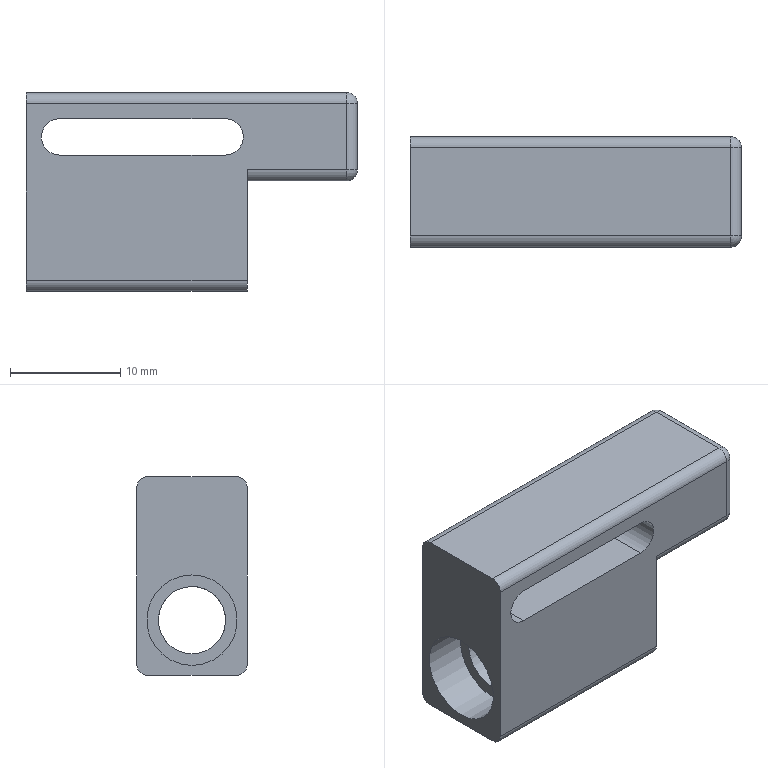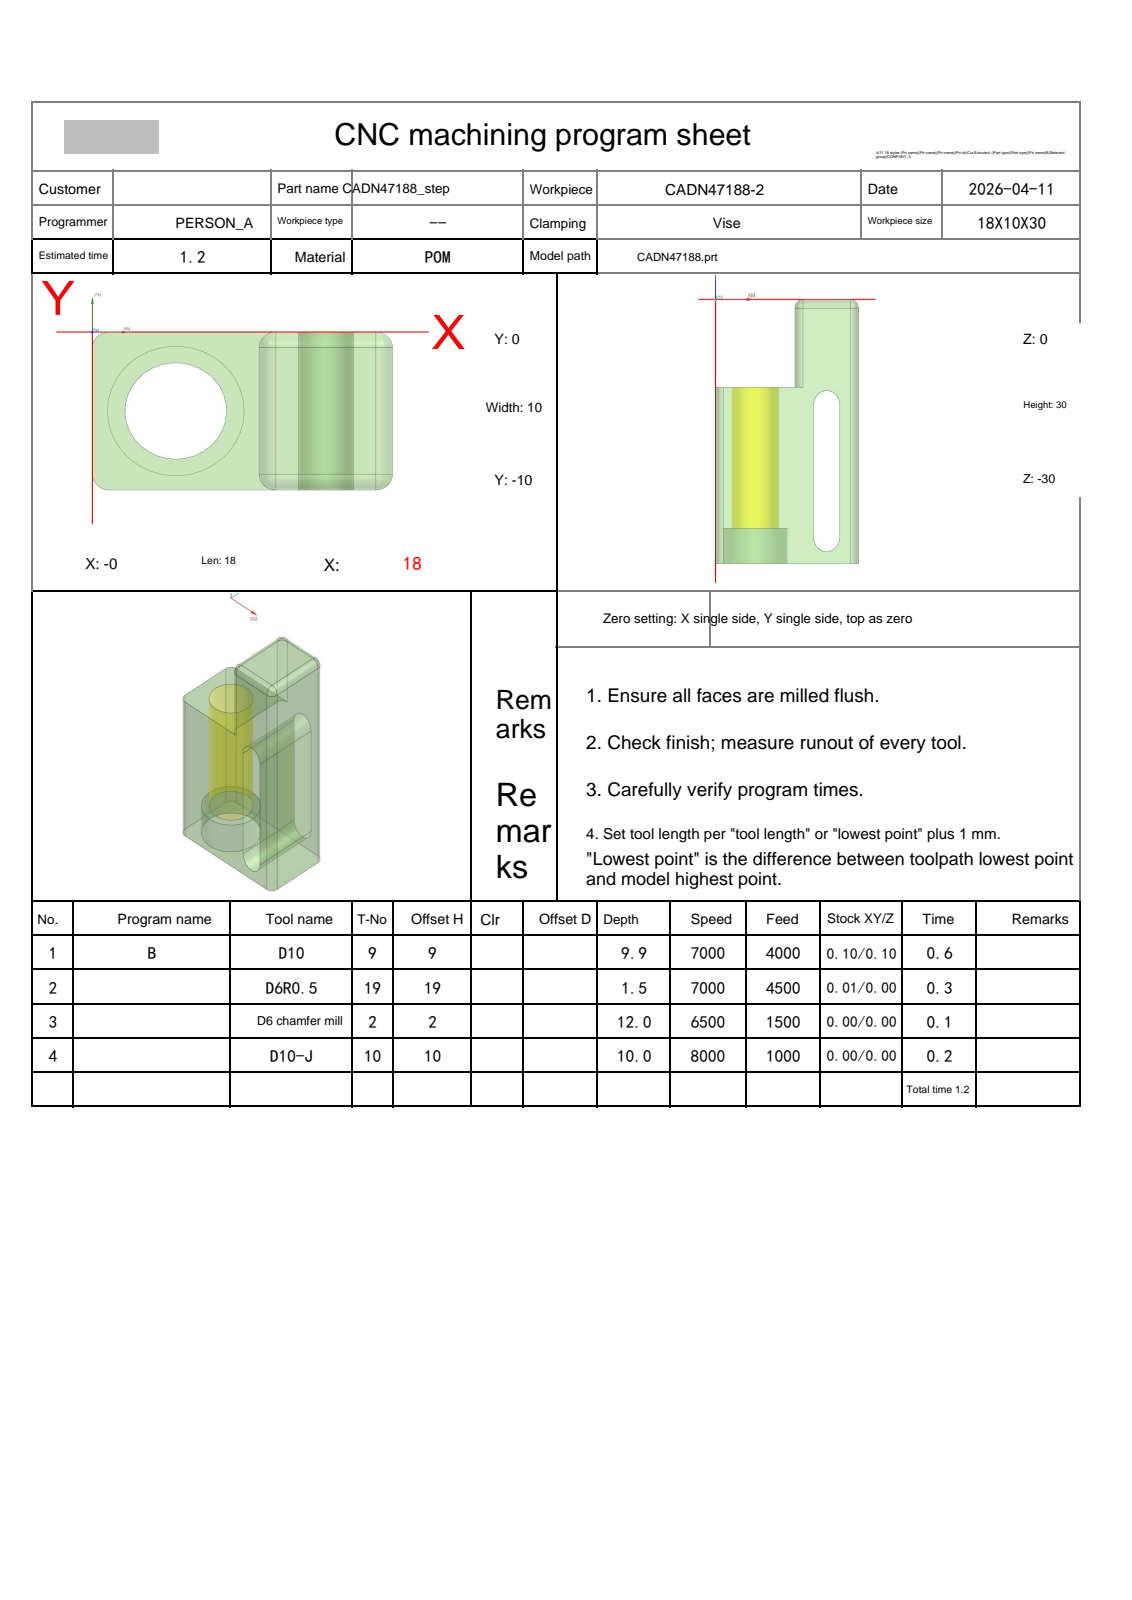NC program | NX | posted by the shop | part box 30 x 10 x 18 mm
Lines 457 to 1926 of 3974:
N2 T19 M06
(D6R0.5  D=6. R=0.5 H=19 ce=0.01 di=0.00)
G00 G90 G54 X13.171 Y-11.678 M03 S7000
G43 H19 Z20.
M08
Z1.5
G01 X10.836 Z1.378 F4500.
X10.409 Y-11.617 Z1.355
X9.997 Y-11.489 Z1.332
X9.611 Y-11.296 Z1.31
X9.261 Y-11.044 Z1.287
X8.956 Y-10.739 Z1.265
X8.704 Y-10.389 Z1.242
X8.511 Y-10.003 Z1.219
X8.383 Y-9.591 Z1.197
X8.322 Y-9.164 Z1.174
Y-.836 Z.738
X8.383 Y-.409 Z.715
X8.511 Y.003 Z.692
X8.704 Y.389 Z.67
X8.956 Y.739 Z.647
X9.261 Y1.044 Z.625
X9.611 Y1.296 Z.602
X9.997 Y1.489 Z.579
X10.409 Y1.617 Z.557
X10.836 Y1.678 Z.534
X17.164 Z.203
X17.591 Y1.617 Z.18
X18.003 Y1.489 Z.157
X18.389 Y1.296 Z.135
X18.739 Y1.044 Z.112
X19.044 Y.739 Z.09
X19.296 Y.389 Z.067
X19.489 Y.003 Z.044
X19.617 Y-.409 Z.022
X19.678 Y-.836 Z-.001
Y-1. Z-.009
Y-9.
G02 X17. Y-11.678 I-2.678 J0.0
G01 X11.
G02 X8.322 Y-9. I0.0 J2.678
G01 Y-1.
G02 X11. Y1.678 I2.678 J0.0
G01 X17.
G02 X19.678 Y-1. I0.0 J-2.678
G01 X19.684 Y-3. Z-.01
X19.69 Y-5. Z-.011
X19.695 Y-7. Z-.012
X19.701 Y-9.
X19.7 Y-9.082
X19.696 Y-9.163
X19.691 Y-9.245
X19.682 Y-9.326
X19.672 Y-9.407
X19.658 Y-9.487
X19.643 Y-9.567
X19.624 Y-9.647
X19.604 Y-9.726 Z-.013
X19.581 Y-9.804
X19.556 Y-9.882
X19.528 Y-9.959
X19.498 Y-10.035
X19.466 Y-10.11
X19.432 Y-10.184
X19.394 Y-10.257
X19.356 Y-10.329
X19.315 Y-10.399
X19.272 Y-10.469
X19.226 Y-10.537
X19.179 Y-10.604
X19.13 Y-10.668
X19.079 Y-10.733
X19.025 Y-10.794
X18.971 Y-10.855
X18.914 Y-10.914
X18.855 Y-10.971
X18.795 Y-11.026
X18.733 Y-11.08
X18.67 Y-11.131
X18.605 Y-11.181
X18.538 Y-11.228
X18.47 Y-11.274
X18.401 Y-11.317
X18.331 Y-11.359
X18.259 Y-11.398
X18.186 Y-11.436
X18.112 Y-11.47
X18.037 Y-11.503
X17.961 Y-11.533
X17.884 Y-11.562
X17.806 Y-11.587
X17.728 Y-11.611
X17.649 Y-11.631 Z-.014
X17.569 Y-11.651
X17.489 Y-11.666
X17.408 Y-11.68
X17.327 Y-11.691
X17.245 Y-11.701
X17.164 Y-11.706
X17.082 Y-11.711
X17. Y-11.712
X14. Y-11.72 Z-.015
X11. Y-11.727 Z-.016
X10.918 Y-11.726
X10.835 Y-11.723
X10.753 Y-11.717
X10.671 Y-11.708
X10.589 Y-11.697
X10.508 Y-11.684
X10.427 Y-11.668
X10.347 Y-11.65
X10.267 Y-11.629
X10.188 Y-11.606
X10.11 Y-11.58
X10.032 Y-11.552
X9.955 Y-11.522
X9.88 Y-11.49
X9.805 Y-11.455
X9.731 Y-11.418
X9.659 Y-11.378
X9.587 Y-11.337
X9.517 Y-11.293
X9.448 Y-11.248
X9.381 Y-11.2
X9.315 Y-11.15
X9.251 Y-11.099 Z-.017
X9.188 Y-11.045
X9.127 Y-10.989
X9.068 Y-10.932
X9.01 Y-10.873
X8.954 Y-10.812
X8.901 Y-10.75
X8.848 Y-10.686
X8.798 Y-10.62
X8.75 Y-10.553
X8.704 Y-10.484
X8.66 Y-10.414
X8.619 Y-10.343
X8.579 Y-10.271
X8.541 Y-10.197
X8.506 Y-10.122
X8.473 Y-10.047
X8.443 Y-9.97
X8.414 Y-9.892
X8.389 Y-9.814
X8.365 Y-9.735
X8.344 Y-9.655
X8.325 Y-9.574
X8.309 Y-9.493
X8.295 Y-9.412
X8.284 Y-9.33
X8.274 Y-9.248
X8.268 Y-9.165
X8.264 Y-9.083
X8.263 Y-9.
X8.259 Y-7. Z-.018
X8.254 Y-5. Z-.019
X8.249 Y-3.
X8.246 Y-1. Z-.02
Y-.917
X8.25 Y-.834
X8.256 Y-.751
X8.265 Y-.668
X8.276 Y-.585
X8.29 Y-.503
X8.305 Y-.422
X8.324 Y-.34
X8.345 Y-.26
X8.369 Y-.18
X8.394 Y-.101
X8.423 Y-.023 Z-.021
X8.453 Y.055
X8.486 Y.131
X8.521 Y.207
X8.559 Y.281
X8.598 Y.355
X8.64 Y.427
X8.684 Y.498
X8.73 Y.567
X8.778 Y.635
X8.829 Y.701
X8.881 Y.766
X8.935 Y.829
X8.991 Y.891
X9.049 Y.951
X9.108 Y1.009
X9.17 Y1.065
X9.233 Y1.12
X9.298 Y1.172
X9.364 Y1.223
X9.432 Y1.272
X9.501 Y1.318
X9.572 Y1.362
X9.644 Y1.405
X9.717 Y1.445
X9.791 Y1.483
X9.867 Y1.518
X9.943 Y1.552
X10.021 Y1.582
X10.099 Y1.611
X10.178 Y1.637
X10.258 Y1.661
X10.339 Y1.682
X10.42 Y1.701
X10.502 Y1.717 Z-.022
X10.584 Y1.732
X10.667 Y1.743
X10.75 Y1.752
X10.833 Y1.758
X10.917 Y1.763
X11. Y1.764
X14. Y1.77 Z-.023
X17. Y1.776 Z-.024
X17.084 Y1.775
X17.168 Y1.771
X17.251 Y1.765
X17.335 Y1.756
X17.418 Y1.745
X17.5 Y1.731
X17.583 Y1.715
X17.665 Y1.696
X17.746 Y1.675
X17.826 Y1.651
X17.906 Y1.626
X17.985 Y1.597
X18.063 Y1.567
X18.14 Y1.533
X18.216 Y1.498
X18.291 Y1.46
X18.365 Y1.42
X18.437 Y1.378
X18.509 Y1.334
X18.579 Y1.287
X18.647 Y1.239
X18.714 Y1.188
X18.78 Y1.135
X18.843 Y1.08
X18.905 Y1.024 Z-.025
X18.966 Y.966
X19.024 Y.906
X19.081 Y.843
X19.136 Y.78
X19.189 Y.715
X19.24 Y.648
X19.288 Y.58
X19.336 Y.51
X19.38 Y.439
X19.423 Y.366
X19.463 Y.293
X19.501 Y.218
X19.537 Y.142
X19.57 Y.065
X19.601 Y-.014
X19.63 Y-.092
X19.656 Y-.172
X19.681 Y-.253
X19.702 Y-.334
X19.721 Y-.416
X19.737 Y-.498
X19.752 Y-.581
X19.763 Y-.665
X19.772 Y-.748
X19.778 Y-.832
X19.783 Y-.916
X19.784 Y-1.
X19.789 Y-3. Z-.026
X19.795 Y-5. Z-.027
X19.8 Y-7. Z-.028
X19.804 Y-9. Z-.029
X19.8 Y-9.157
X19.787 Y-9.314
X19.766 Y-9.47
X19.735 Y-9.624 Z-.03
X19.697 Y-9.777
X19.649 Y-9.927
X19.593 Y-10.074
X19.529 Y-10.218
X19.457 Y-10.358
X19.378 Y-10.494
X19.291 Y-10.625
X19.196 Y-10.751
X19.095 Y-10.872
X18.987 Y-10.987
X18.872 Y-11.095
X18.752 Y-11.197
X18.627 Y-11.292 Z-.031
X18.496 Y-11.38
X18.36 Y-11.461
X18.22 Y-11.533
X18.076 Y-11.598
X17.929 Y-11.655
X17.779 Y-11.703
X17.626 Y-11.743
X17.471 Y-11.774
X17.315 Y-11.796
X17.158 Y-11.81
X17. Y-11.815
X14. Y-11.822 Z-.033
X11. Y-11.829 Z-.034
X10.841 Y-11.825
X10.683 Y-11.812
X10.526 Y-11.79 Z-.035
X10.37 Y-11.759
X10.216 Y-11.72
X10.065 Y-11.672
X9.917 Y-11.616
X9.771 Y-11.551
X9.63 Y-11.479
X9.493 Y-11.398
X9.361 Y-11.31
X9.234 Y-11.215
X9.112 Y-11.113
X8.996 Y-11.004
X8.887 Y-10.888
X8.784 Y-10.767 Z-.036
X8.688 Y-10.64
X8.599 Y-10.509
X8.518 Y-10.372
X8.445 Y-10.231
X8.38 Y-10.085
X8.322 Y-9.937
X8.274 Y-9.785
X8.234 Y-9.631
X8.203 Y-9.475
X8.18 Y-9.318
X8.166 Y-9.159
X8.161 Y-9.
X8.157 Y-7. Z-.037
X8.153 Y-5. Z-.038
X8.149 Y-3. Z-.039
X8.145 Y-1. Z-.04
X8.149 Y-.84
X8.162 Y-.68 Z-.041
X8.184 Y-.521
X8.215 Y-.364
X8.254 Y-.209
X8.303 Y-.056
X8.36 Y.094
X8.425 Y.24
X8.498 Y.383
X8.58 Y.521
X8.668 Y.655
X8.764 Y.783
X8.868 Y.906
X8.978 Y1.022 Z-.042
X9.094 Y1.133
X9.216 Y1.237
X9.344 Y1.333
X9.478 Y1.423
X9.616 Y1.505
X9.758 Y1.579
X9.905 Y1.645
X10.055 Y1.702
X10.207 Y1.751
X10.363 Y1.792
X10.52 Y1.823
X10.679 Y1.846
X10.839 Y1.86 Z-.043
X11. Y1.865
X14. Y1.871 Z-.044
X17. Y1.877 Z-.046
X17.161 Y1.872
X17.322 Y1.859
X17.482 Y1.837
X17.64 Y1.806
X17.797 Y1.766
X17.951 Y1.717
X18.102 Y1.66
X18.249 Y1.594
X18.393 Y1.52
X18.532 Y1.438
X18.667 Y1.349
X18.796 Y1.252
X18.92 Y1.148 Z-.047
X19.037 Y1.037
X19.148 Y.92
X19.253 Y.797
X19.35 Y.668
X19.44 Y.533
X19.523 Y.394
X19.597 Y.251
X19.664 Y.103
X19.721 Y-.048
X19.771 Y-.202
X19.812 Y-.358
X19.844 Y-.517 Z-.048
X19.866 Y-.677
X19.88 Y-.838
X19.886 Y-1.
X19.89 Y-3. Z-.049
X19.895 Y-5. Z-.05
X19.899 Y-7. Z-.051
X19.904 Y-9. Z-.053
X19.9 Y-9.163
X19.886 Y-9.325
X19.864 Y-9.487
X19.833 Y-9.647
X19.792 Y-9.804
X19.743 Y-9.96
X19.685 Y-10.112
X19.619 Y-10.261 Z-.054
X19.545 Y-10.406
X19.462 Y-10.547
X19.372 Y-10.683
X19.274 Y-10.813
X19.169 Y-10.938
X19.057 Y-11.057
X18.939 Y-11.169
X18.814 Y-11.275
X18.684 Y-11.373
X18.548 Y-11.464 Z-.055
X18.408 Y-11.548
X18.263 Y-11.623
X18.114 Y-11.69
X17.962 Y-11.748
X17.806 Y-11.799
X17.648 Y-11.84
X17.488 Y-11.872
X17.326 Y-11.895
X17.163 Y-11.909
X17. Y-11.914 Z-.056
X14. Y-11.921 Z-.057
X11. Y-11.927 Z-.059
X10.836 Y-11.923
X10.672 Y-11.91
X10.509 Y-11.887 Z-.06
X10.348 Y-11.855
X10.189 Y-11.815
X10.032 Y-11.765
X9.879 Y-11.707
X9.729 Y-11.64
X9.582 Y-11.565
X9.441 Y-11.482
X9.304 Y-11.391
X9.172 Y-11.292 Z-.061
X9.046 Y-11.186
X8.927 Y-11.073
X8.813 Y-10.954
X8.707 Y-10.829
X8.608 Y-10.697
X8.516 Y-10.561
X8.432 Y-10.419
X8.356 Y-10.273
X8.289 Y-10.123
X8.23 Y-9.969 Z-.062
X8.179 Y-9.813
X8.138 Y-9.653
X8.105 Y-9.492
X8.082 Y-9.329
X8.068 Y-9.165
X8.063 Y-9.
X8.059 Y-7. Z-.063
X8.055 Y-5. Z-.065
X8.051 Y-3. Z-.066
X8.047 Y-1. Z-.067
X8.051 Y-.834
X8.065 Y-.669
X8.087 Y-.505
X8.12 Y-.343 Z-.068
X8.16 Y-.182
X8.211 Y-.024
X8.269 Y.131
X8.337 Y.283
X8.413 Y.43
X8.497 Y.573
X8.588 Y.711
X8.688 Y.844
X8.795 Y.971
X8.908 Y1.092 Z-.069
X9.029 Y1.206
X9.155 Y1.313
X9.288 Y1.413
X9.426 Y1.506
X9.568 Y1.59
X9.716 Y1.667
X9.867 Y1.735
X10.022 Y1.794
X10.18 Y1.845
X10.341 Y1.887 Z-.07
X10.504 Y1.92
X10.668 Y1.943
X10.834 Y1.958
X11. Y1.963
X14. Y1.968 Z-.072
X17. Y1.974 Z-.074
X17.167 Y1.97
X17.333 Y1.956
X17.498 Y1.933
X17.662 Y1.901
X17.824 Y1.86
X17.983 Y1.809
X18.139 Y1.75
X18.292 Y1.682 Z-.075
X18.44 Y1.606
X18.584 Y1.521
X18.723 Y1.428
X18.857 Y1.328
X18.985 Y1.221
X19.106 Y1.106
X19.221 Y.985
X19.329 Y.858
X19.43 Y.724
X19.523 Y.585 Z-.076
X19.608 Y.442
X19.685 Y.293
X19.754 Y.141
X19.814 Y-.015
X19.865 Y-.175
X19.907 Y-.337
X19.94 Y-.5
X19.964 Y-.666
X19.978 Y-.833 Z-.077
X19.983 Y-1.
X19.987 Y-3. Z-.078
X19.992 Y-5. Z-.08
X19.997 Y-7. Z-.081
X20.001 Y-9. Z-.083
X19.996 Y-9.168
X19.982 Y-9.336
X19.959 Y-9.503
X19.927 Y-9.668
X19.885 Y-9.831
X19.834 Y-9.992
X19.775 Y-10.149
X19.706 Y-10.303 Z-.084
X19.629 Y-10.453
X19.544 Y-10.598
X19.45 Y-10.739
X19.349 Y-10.874
X19.241 Y-11.003
X19.125 Y-11.125
X19.003 Y-11.241
X18.874 Y-11.35 Z-.085
X18.74 Y-11.452
X18.6 Y-11.546
X18.455 Y-11.632
X18.305 Y-11.71
X18.151 Y-11.779
X17.994 Y-11.84
X17.833 Y-11.891
X17.67 Y-11.934 Z-.086
X17.504 Y-11.967
X17.337 Y-11.991
X17.169 Y-12.006
X17. Y-12.011
X14. Y-12.017 Z-.088
X11. Y-12.023 Z-.091
X10.83 Y-12.019
X10.661 Y-12.005
X10.493 Y-11.982
X10.327 Y-11.949
X10.163 Y-11.907
X10.001 Y-11.856
X9.842 Y-11.795
X9.687 Y-11.726 Z-.092
X9.536 Y-11.649
X9.39 Y-11.563
X9.248 Y-11.469
X9.112 Y-11.367
X8.982 Y-11.258
X8.859 Y-11.141
X8.742 Y-11.018
X8.632 Y-10.888 Z-.093
X8.53 Y-10.753
X8.435 Y-10.612
X8.348 Y-10.466
X8.27 Y-10.315
X8.2 Y-10.16
X8.139 Y-10.001
X8.087 Y-9.839 Z-.094
X8.044 Y-9.675
X8.011 Y-9.508
X7.987 Y-9.34
X7.972 Y-9.17
X7.967 Y-9.
X7.963 Y-7. Z-.096
X7.959 Y-5. Z-.097
X7.955 Y-3. Z-.099
X7.952 Y-1. Z-.1
X7.956 Y-.829
X7.97 Y-.659
X7.993 Y-.489 Z-.101
X8.027 Y-.321
X8.069 Y-.156
X8.121 Y.008
X8.181 Y.168
X8.251 Y.324
X8.329 Y.476
X8.416 Y.624
X8.511 Y.766 Z-.102
X8.613 Y.903
X8.724 Y1.034
X8.841 Y1.159
X8.965 Y1.277
X9.096 Y1.388
X9.233 Y1.491
X9.375 Y1.586
X9.522 Y1.674 Z-.103
X9.674 Y1.753
X9.831 Y1.823
X9.991 Y1.884
X10.154 Y1.937
X10.32 Y1.98
X10.488 Y2.014
X10.658 Y2.038
X10.829 Y2.053 Z-.104
X11. Y2.058
X14. Y2.063 Z-.106
X17. Y2.069 Z-.108
X17.172 Y2.065
X17.344 Y2.051
X17.514 Y2.027 Z-.109
X17.683 Y1.994
X17.85 Y1.951
X18.014 Y1.899
X18.175 Y1.838
X18.333 Y1.768
X18.486 Y1.689
X18.635 Y1.601
X18.778 Y1.506 Z-.11
X18.916 Y1.403
X19.048 Y1.292
X19.173 Y1.173
X19.292 Y1.048
X19.404 Y.917
X19.507 Y.779
X19.604 Y.636 Z-.111
X19.691 Y.488
X19.771 Y.334
X19.842 Y.177
X19.903 Y.016
X19.956 Y-.148
X20. Y-.315
X20.034 Y-.485
X20.058 Y-.655 Z-.112
X20.073 Y-.827
X20.078 Y-1.
X20.082 Y-3. Z-.114
X20.087 Y-5. Z-.115
X20.09 Y-7. Z-.117
X20.095 Y-9. Z-.119
X20.09 Y-9.174
X20.076 Y-9.347
X20.052 Y-9.519
X20.018 Y-9.689
X19.975 Y-9.857
X19.923 Y-10.023 Z-.12
X19.861 Y-10.185
X19.791 Y-10.344
X19.711 Y-10.499
X19.623 Y-10.648
X19.527 Y-10.793
X19.423 Y-10.932 Z-.121
X19.311 Y-11.065
X19.192 Y-11.192
X19.066 Y-11.311
X18.933 Y-11.424
X18.794 Y-11.529
X18.65 Y-11.626
X18.5 Y-11.714 Z-.122
X18.346 Y-11.794
X18.187 Y-11.866
X18.025 Y-11.928
X17.859 Y-11.982
X17.69 Y-12.025
X17.605 Y-12.044
X17.52 Y-12.06
X17.434 Y-12.073 Z-.123
X17.348 Y-12.084
X17.261 Y-12.093
X17.174 Y-12.099
X17.087 Y-12.103
X17. Y-12.104
X14. Y-12.11 Z-.126
X11. Y-12.116 Z-.128
X10.825 Y-12.112
X10.651 Y-12.098
X10.478 Y-12.073 Z-.129
X10.306 Y-12.04
X10.137 Y-11.996
X9.97 Y-11.944
X9.806 Y-11.881
X9.647 Y-11.81
X9.491 Y-11.73 Z-.13
X9.34 Y-11.642
X9.194 Y-11.545
X9.054 Y-11.44
X8.92 Y-11.327
X8.793 Y-11.207
X8.672 Y-11.08
X8.559 Y-10.947 Z-.131
X8.454 Y-10.807
X8.356 Y-10.661
X8.267 Y-10.511
X8.186 Y-10.355
X8.114 Y-10.195
X8.051 Y-10.032
X7.998 Y-9.865 Z-.132
X7.954 Y-9.695
X7.919 Y-9.523
X7.894 Y-9.35
X7.879 Y-9.175
X7.874 Y-9.
X7.87 Y-7. Z-.134
X7.866 Y-5. Z-.136
X7.863 Y-3. Z-.138
X7.859 Y-1. Z-.139
X7.86 Y-.912
X7.863 Y-.824
X7.869 Y-.736 Z-.14
X7.878 Y-.648
X7.889 Y-.561
X7.902 Y-.474
X7.918 Y-.387
X7.936 Y-.301
X7.957 Y-.215
X7.98 Y-.13
X8.005 Y-.046
X8.033 Y.038
X8.063 Y.121
X8.096 Y.203
X8.131 Y.284
X8.168 Y.364 Z-.141
X8.207 Y.443
X8.248 Y.521
X8.292 Y.598
X8.338 Y.673
X8.385 Y.747
X8.435 Y.82
X8.487 Y.891
X8.541 Y.961
X8.597 Y1.029
X8.655 Y1.096
X8.714 Y1.161
X8.776 Y1.224
X8.839 Y1.286 Z-.142
X8.904 Y1.346
X8.97 Y1.404
X9.038 Y1.46
X9.108 Y1.514
X9.179 Y1.566
X9.252 Y1.617
X9.326 Y1.665
X9.401 Y1.711
X9.478 Y1.755
X9.555 Y1.796
X9.634 Y1.836
X9.714 Y1.873
X9.795 Y1.908 Z-.143
X9.877 Y1.941
X9.96 Y1.972
X10.044 Y2.
X10.128 Y2.026
X10.213 Y2.049
X10.299 Y2.07
X10.386 Y2.089
X10.472 Y2.105
X10.56 Y2.119
X10.647 Y2.13
X10.735 Y2.139
X10.823 Y2.145
X10.912 Y2.149 Z-.144
X11. Y2.15
X14. Y2.156 Z-.146
X17. Y2.161 Z-.149
X17.177 Y2.157
X17.354 Y2.142
X17.53 Y2.117
X17.704 Y2.083
X17.876 Y2.039 Z-.15
X18.045 Y1.986
X18.211 Y1.923
X18.373 Y1.851
X18.531 Y1.769
X18.684 Y1.679
X18.831 Y1.581 Z-.151
X18.973 Y1.475
X19.109 Y1.36
X19.238 Y1.238
X19.361 Y1.11
X19.476 Y.974
X19.583 Y.832
X19.681 Y.685 Z-.152
X19.772 Y.532
X19.854 Y.374
X19.927 Y.212
X19.99 Y.046
X20.045 Y-.123
X20.089 Y-.295 Z-.153
X20.108 Y-.382
X20.124 Y-.469
X20.138 Y-.557
X20.149 Y-.645
X20.165 Y-.822
X20.17 Y-1.
X20.174 Y-3. Z-.155
X20.178 Y-5. Z-.157
X20.182 Y-7. Z-.159
X20.186 Y-9. Z-.161
X20.185 Y-9.089
X20.181 Y-9.179
X20.175 Y-9.268
X20.166 Y-9.357
X20.156 Y-9.445
X20.142 Y-9.534
X20.126 Y-9.622 Z-.162
X20.107 Y-9.709
X20.086 Y-9.796
X20.063 Y-9.882
X20.037 Y-9.968
X20.009 Y-10.053
X19.979 Y-10.137
X19.946 Y-10.22
X19.91 Y-10.302
X19.873 Y-10.383
X19.833 Y-10.464
X19.791 Y-10.543 Z-.163
X19.747 Y-10.62
X19.7 Y-10.697
X19.652 Y-10.772
X19.601 Y-10.846
X19.549 Y-10.918
X19.494 Y-10.989
X19.437 Y-11.058
X19.379 Y-11.126
X19.318 Y-11.192
X19.256 Y-11.256
X19.192 Y-11.319 Z-.164
X19.126 Y-11.379
X19.059 Y-11.438
X18.99 Y-11.495
X18.919 Y-11.55
X18.847 Y-11.603
X18.773 Y-11.654
X18.698 Y-11.703
X18.622 Y-11.75
X18.544 Y-11.794
X18.465 Y-11.837
X18.385 Y-11.876
X18.304 Y-11.915 Z-.165
X18.222 Y-11.95
X18.139 Y-11.983
X18.055 Y-12.014
X17.97 Y-12.043
X17.884 Y-12.069
X17.798 Y-12.093
X17.711 Y-12.114
X17.623 Y-12.133
X17.535 Y-12.149
X17.447 Y-12.163
X17.358 Y-12.175 Z-.166
X17.269 Y-12.184
X17.179 Y-12.19
X17.09 Y-12.194
X17. Y-12.195
X14. Y-12.201 Z-.169
X11. Y-12.207 Z-.172
X10.91 Y-12.206
X10.82 Y-12.202
X10.73 Y-12.196
X10.641 Y-12.187
X10.552 Y-12.176
X10.463 Y-12.162
X10.374 Y-12.146
X10.286 Y-12.128
X10.199 Y-12.107 Z-.173
X10.112 Y-12.083
X10.026 Y-12.057
X9.94 Y-12.029
X9.856 Y-11.998
X9.772 Y-11.965
X9.689 Y-11.93
X9.607 Y-11.892
X9.527 Y-11.852
X9.447 Y-11.809
X9.369 Y-11.765
X9.292 Y-11.718 Z-.174
X9.216 Y-11.669
X9.142 Y-11.618
X9.069 Y-11.565
X8.998 Y-11.51
X8.928 Y-11.453
X8.86 Y-11.394
X8.794 Y-11.334
X8.729 Y-11.271
X8.666 Y-11.206
X8.605 Y-11.14
X8.546 Y-11.072
X8.489 Y-11.003 Z-.175
X8.433 Y-10.932
X8.38 Y-10.859
X8.329 Y-10.785
X8.28 Y-10.709
X8.233 Y-10.632
X8.188 Y-10.554
X8.145 Y-10.475
X8.105 Y-10.394
X8.067 Y-10.313
X8.031 Y-10.23
X7.997 Y-10.146 Z-.176
X7.966 Y-10.062
X7.937 Y-9.976
X7.911 Y-9.89
X7.887 Y-9.803
X7.866 Y-9.715
X7.847 Y-9.627
X7.83 Y-9.539
X7.816 Y-9.449
X7.805 Y-9.36
X7.796 Y-9.27
X7.789 Y-9.18 Z-.177
X7.785 Y-9.09
X7.784 Y-9.
X7.78 Y-7. Z-.179
X7.777 Y-5. Z-.181
X7.773 Y-3. Z-.183
X7.769 Y-1. Z-.185
X7.77 Y-.909
X7.774 Y-.819
X7.78 Y-.728
X7.789 Y-.638
X7.8 Y-.548
X7.814 Y-.459
X7.83 Y-.369
X7.849 Y-.281
X7.87 Y-.193
X7.894 Y-.105
X7.92 Y-.018 Z-.186
X7.949 Y.068
X7.98 Y.153
X8.013 Y.237
X8.049 Y.321
X8.087 Y.403
X8.127 Y.484
X8.17 Y.564
X8.215 Y.643
X8.262 Y.72
X8.311 Y.797
X8.362 Y.871 Z-.187
X8.416 Y.945
X8.471 Y1.017
X8.528 Y1.087
X8.588 Y1.155
X8.649 Y1.223
X8.712 Y1.288
X8.777 Y1.351
X8.844 Y1.412
X8.912 Y1.472
X8.983 Y1.53
X9.054 Y1.586
X9.127 Y1.639 Z-.188
X9.202 Y1.691
X9.278 Y1.74
X9.356 Y1.788
X9.434 Y1.833
X9.514 Y1.876
X9.596 Y1.916
X9.678 Y1.955
X9.761 Y1.991
X9.845 Y2.025
X9.931 Y2.056
X10.017 Y2.085 Z-.189
X10.104 Y2.111
X10.191 Y2.136
X10.279 Y2.157
X10.368 Y2.176
X10.458 Y2.193
X10.547 Y2.207
X10.637 Y2.219
X10.728 Y2.228
X10.818 Y2.234
X10.909 Y2.238
X11. Y2.24 Z-.19
X14. Y2.245 Z-.192
X17. Y2.25 Z-.195
X17.091 Y2.249 Z-.196
X17.182 Y2.245
X17.273 Y2.239
X17.364 Y2.23
X17.454 Y2.219
X17.545 Y2.205
X17.634 Y2.189
X17.724 Y2.17
X17.812 Y2.149
X17.9 Y2.125
X17.988 Y2.098
X18.074 Y2.07
X18.16 Y2.038 Z-.197
X18.245 Y2.005
X18.329 Y1.969
X18.411 Y1.931
X18.493 Y1.89
X18.574 Y1.847
X18.653 Y1.802
X18.731 Y1.755
X18.808 Y1.705
X18.883 Y1.654
X18.957 Y1.6
X19.029 Y1.544 Z-.198
X19.1 Y1.486
X19.168 Y1.427
X19.236 Y1.365
X19.301 Y1.301
X19.365 Y1.236
X19.427 Y1.169
X19.487 Y1.1
X19.545 Y1.03
X19.601 Y.958
X19.655 Y.884
X19.707 Y.809 Z-.199
X19.757 Y.732
X19.804 Y.654
X19.85 Y.575
X19.893 Y.495
X19.934 Y.413
X19.973 Y.33
X20.009 Y.246
X20.043 Y.162
X20.074 Y.076
X20.103 Y-.011
X20.13 Y-.098 Z-.2
X20.154 Y-.186
X20.176 Y-.275
X20.195 Y-.364
X20.212 Y-.454
X20.226 Y-.545
X20.238 Y-.635
X20.247 Y-.726
X20.253 Y-.817
X20.258 Y-.909
X20.259 Y-1.
X20.262 Y-3. Z-.203
X20.267 Y-5. Z-.205
X20.27 Y-7. Z-.207
X20.274 Y-9. Z-.209
X20.27 Y-9.171
X20.256 Y-9.342
X20.234 Y-9.512 Z-.21
X20.203 Y-9.681
X20.164 Y-9.848
X20.115 Y-10.012
X20.058 Y-10.174
X19.993 Y-10.333 Z-.211
X19.919 Y-10.488
X19.838 Y-10.638
X19.749 Y-10.785
X19.652 Y-10.926
X19.547 Y-11.063 Z-.212
X19.436 Y-11.193
X19.318 Y-11.318
X19.194 Y-11.437
X19.064 Y-11.548
X18.928 Y-11.653
X18.786 Y-11.751 Z-.213
X18.64 Y-11.841
X18.489 Y-11.923
X18.334 Y-11.997
X18.176 Y-12.063
X18.014 Y-12.121 Z-.214
X17.849 Y-12.17
X17.682 Y-12.21
X17.513 Y-12.242
X17.343 Y-12.264
X17.172 Y-12.278 Z-.215
X17. Y-12.283
X14. Y-12.289 Z-.218
X11. Y-12.294 Z-.221
X10.828 Y-12.29
X10.656 Y-12.276 Z-.222
X10.485 Y-12.254
X10.315 Y-12.223
X10.147 Y-12.183
X9.982 Y-12.134
X9.819 Y-12.077 Z-.223
X9.659 Y-12.011
X9.503 Y-11.937
X9.351 Y-11.855
X9.204 Y-11.765
X9.062 Y-11.668 Z-.224
X8.925 Y-11.563
X8.793 Y-11.451
X8.668 Y-11.332
X8.548 Y-11.207
X8.436 Y-11.076
X8.331 Y-10.939 Z-.225
X8.233 Y-10.797
X8.142 Y-10.65
X8.059 Y-10.498
X7.985 Y-10.343
X7.918 Y-10.183 Z-.226
X7.86 Y-10.02
X7.811 Y-9.854
X7.77 Y-9.687
X7.739 Y-9.517
X7.716 Y-9.345 Z-.227
X7.702 Y-9.173
X7.697 Y-9.
X7.693 Y-7. Z-.229
X7.69 Y-5. Z-.231
X7.687 Y-3. Z-.233
X7.683 Y-1. Z-.236
X7.687 Y-.826
X7.701 Y-.653
X7.723 Y-.481
X7.755 Y-.31
X7.795 Y-.141 Z-.237
X7.844 Y.025
X7.902 Y.189
X7.968 Y.35
X8.042 Y.507
X8.125 Y.66
X8.216 Y.808 Z-.238
X8.314 Y.952
X8.419 Y1.09
X8.532 Y1.222
X8.652 Y1.348
X8.778 Y1.468 Z-.239
X8.91 Y1.582
X9.047 Y1.688
X9.19 Y1.786
X9.339 Y1.877
X9.491 Y1.961 Z-.24
X9.648 Y2.036
X9.809 Y2.103
X9.973 Y2.161
X10.14 Y2.211
X10.309 Y2.252 Z-.241
X10.48 Y2.284
X10.652 Y2.307
X10.826 Y2.321
X11. Y2.326
X14. Y2.331 Z-.245
X17. Y2.336 Z-.248
X17.175 Y2.331
X17.349 Y2.318
X17.522 Y2.295
X17.694 Y2.264 Z-.249
X17.864 Y2.223
X18.031 Y2.174
X18.196 Y2.116
X18.358 Y2.05
X18.516 Y1.974
X18.669 Y1.891 Z-.25
X18.818 Y1.8
X18.963 Y1.701
X19.102 Y1.595
X19.235 Y1.482
X19.362 Y1.362 Z-.251
X19.482 Y1.235
X19.596 Y1.102
X19.703 Y.964
X19.802 Y.82
X19.894 Y.671 Z-.252
X19.977 Y.517
X20.053 Y.359
X20.12 Y.198
X20.179 Y.033
X20.229 Y-.135 Z-.253
X20.27 Y-.305
X20.302 Y-.477
X20.325 Y-.65
X20.339 Y-.825
X20.344 Y-1.
X20.348 Y-3. Z-.256
X20.351 Y-5. Z-.258
X20.355 Y-7. Z-.261
X20.358 Y-9. Z-.263
X20.354 Y-9.176
X20.34 Y-9.351
X20.318 Y-9.526 Z-.264
X20.286 Y-9.698
X20.245 Y-9.87
X20.196 Y-10.038
X20.137 Y-10.204
X20.07 Y-10.367 Z-.265
X19.995 Y-10.526
X19.911 Y-10.681
X19.819 Y-10.831
X19.72 Y-10.976 Z-.266
X19.613 Y-11.116
X19.499 Y-11.25
X19.378 Y-11.378
X19.25 Y-11.499
X19.117 Y-11.614 Z-.267
X18.977 Y-11.721
X18.832 Y-11.821
X18.682 Y-11.914
X18.527 Y-11.998
X18.369 Y-12.074 Z-.268
X18.206 Y-12.142
X18.04 Y-12.201
X17.871 Y-12.251
X17.7 Y-12.292
X17.527 Y-12.325 Z-.269
X17.352 Y-12.348
X17.176 Y-12.362
X17. Y-12.367
X14. Y-12.372 Z-.273
X11. Y-12.377 Z-.276
X10.823 Y-12.373 Z-.277
X10.647 Y-12.36
X10.471 Y-12.337
X10.298 Y-12.305
X10.125 Y-12.264
X9.956 Y-12.214 Z-.278
X9.789 Y-12.155
X9.625 Y-12.088
X9.465 Y-12.012
X9.31 Y-11.928 Z-.279
X9.159 Y-11.835
X9.013 Y-11.735
X8.872 Y-11.628
X8.737 Y-11.513
X8.609 Y-11.391 Z-.28
X8.486 Y-11.263
X8.371 Y-11.129
X8.263 Y-10.988
X8.163 Y-10.843
X8.07 Y-10.692 Z-.281
X7.985 Y-10.536
X7.908 Y-10.376
X7.841 Y-10.213
X7.781 Y-10.046
X7.73 Y-9.876 Z-.282
X7.689 Y-9.704
X7.656 Y-9.53
X7.633 Y-9.354
X7.619 Y-9.177 Z-.283
X7.614 Y-9.
X7.61 Y-7. Z-.285
X7.607 Y-5. Z-.287
X7.604 Y-3. Z-.29
X7.601 Y-1. Z-.292
X7.605 Y-.822
X7.619 Y-.645 Z-.293
X7.642 Y-.468
X7.674 Y-.293
X7.715 Y-.12
X7.765 Y.051
X7.825 Y.219 Z-.294
X7.893 Y.384
X7.969 Y.544
X8.054 Y.701
X8.146 Y.853 Z-.295
X8.247 Y1.
X8.355 Y1.142
X8.471 Y1.277
X8.593 Y1.407
X8.722 Y1.53 Z-.296
X8.858 Y1.646
X8.999 Y1.754
X9.146 Y1.856
X9.298 Y1.949
X9.454 Y2.034 Z-.297
X9.615 Y2.111
X9.779 Y2.18
X9.947 Y2.239
X10.118 Y2.29 Z-.298
X10.292 Y2.332
X10.467 Y2.365
X10.644 Y2.389
X10.822 Y2.403
X11. Y2.408 Z-.299
X14. Y2.413 Z-.302
X17. Y2.417 Z-.306
X17.179 Y2.413
X17.357 Y2.399
X17.535 Y2.376
X17.711 Y2.344 Z-.307
X17.885 Y2.302
X18.057 Y2.252
X18.225 Y2.192
X18.391 Y2.124
X18.553 Y2.047 Z-.308
X18.71 Y1.962
X18.863 Y1.869
X19.011 Y1.768
X19.153 Y1.659
X19.289 Y1.543 Z-.309
X19.419 Y1.419
X19.543 Y1.29
X19.659 Y1.154
X19.769 Y1.012 Z-.31
X19.871 Y.864
X19.964 Y.712
X20.05 Y.554
X20.128 Y.393
X20.196 Y.227 Z-.311
X20.257 Y.058
X20.308 Y-.114
X20.35 Y-.288
X20.383 Y-.464
X20.406 Y-.642 Z-.312
X20.421 Y-.821
X20.426 Y-1.
X20.429 Y-3. Z-.315
X20.432 Y-5. Z-.317
X20.436 Y-7. Z-.32
X20.439 Y-9. Z-.322
X20.434 Y-9.18 Z-.323
X20.421 Y-9.36
X20.397 Y-9.538
X20.365 Y-9.715
X20.323 Y-9.89 Z-.324
X20.272 Y-10.063
X20.212 Y-10.233
X20.144 Y-10.4
X20.066 Y-10.562
X19.981 Y-10.721 Z-.325
X19.887 Y-10.875
X19.785 Y-11.023
X19.675 Y-11.167
X19.559 Y-11.304 Z-.326
X19.435 Y-11.435
X19.304 Y-11.559
X19.167 Y-11.676
X19.024 Y-11.786 Z-.327
X18.876 Y-11.889
X18.722 Y-11.983
X18.564 Y-12.07
X18.401 Y-12.147
X18.235 Y-12.217 Z-.328
X18.065 Y-12.277
X17.892 Y-12.329
X17.717 Y-12.371
X17.539 Y-12.404 Z-.329
X17.36 Y-12.428
X17.18 Y-12.443
X17. Y-12.447
X14. Y-12.453 Z-.333
X11. Y-12.457 Z-.337
X10.819 Y-12.453
X10.639 Y-12.439
X10.459 Y-12.415 Z-.338
X10.281 Y-12.383
X10.105 Y-12.341
X9.931 Y-12.29
X9.76 Y-12.229 Z-.339
X9.593 Y-12.16
X9.429 Y-12.083
X9.27 Y-11.996
X9.115 Y-11.902 Z-.34
X8.966 Y-11.8
X8.822 Y-11.69
X8.684 Y-11.572
X8.552 Y-11.448
X8.427 Y-11.316 Z-.341
X8.31 Y-11.179
X8.199 Y-11.035
X8.096 Y-10.886
X8.001 Y-10.731 Z-.342
X7.914 Y-10.572
X7.836 Y-10.409
X7.766 Y-10.241
X7.705 Y-10.07 Z-.343
X7.654 Y-9.897
X7.611 Y-9.72
X7.578 Y-9.542
X7.554 Y-9.362
X7.539 Y-9.181 Z-.344
X7.534 Y-9.
X7.531 Y-7. Z-.347
X7.528 Y-5. Z-.349
X7.525 Y-3. Z-.352
X7.522 Y-1. Z-.354
X7.527 Y-.818
X7.541 Y-.636 Z-.355
X7.564 Y-.456
X7.597 Y-.277
X7.639 Y-.099
X7.691 Y.075 Z-.356
X7.751 Y.247
X7.821 Y.415
X7.899 Y.58
X7.986 Y.74 Z-.357
X8.081 Y.896
X8.184 Y1.046
X8.294 Y1.191
X8.413 Y1.33
X8.538 Y1.462 Z-.358
X8.67 Y1.588
X8.808 Y1.706
X8.953 Y1.818
X9.103 Y1.921 Z-.359
X9.258 Y2.017
X9.418 Y2.104
X9.583 Y2.183
X9.751 Y2.253 Z-.36
X9.923 Y2.314
X10.098 Y2.366
X10.275 Y2.409
X10.455 Y2.442 Z-.361
X10.636 Y2.466
X10.818 Y2.481
X11. Y2.486
X14. Y2.491 Z-.365
X17. Y2.495 Z-.369
X17.183 Y2.49
X17.365 Y2.476
X17.547 Y2.453 Z-.37
X17.727 Y2.42
X17.905 Y2.377
X18.081 Y2.326
X18.253 Y2.265 Z-.371
X18.422 Y2.195
X18.588 Y2.116
X18.749 Y2.029
X18.905 Y1.934
X19.056 Y1.83 Z-.372
X19.202 Y1.719
X19.341 Y1.6
X19.474 Y1.474
X19.601 Y1.342 Z-.373
X19.72 Y1.202
X19.832 Y1.057
X19.935 Y.906
X20.032 Y.75 Z-.374
X20.119 Y.589
X20.198 Y.424
X20.269 Y.255
X20.33 Y.082 Z-.375
X20.382 Y-.094
X20.426 Y-.272
X20.459 Y-.452
X20.483 Y-.634
X20.498 Y-.817 Z-.376
X20.503 Y-1.
X20.506 Y-3. Z-.379
X20.509 Y-5. Z-.381
X20.512 Y-7. Z-.384
X20.515 Y-9. Z-.387
X20.511 Y-9.184
X20.497 Y-9.368
X20.473 Y-9.55 Z-.388
X20.44 Y-9.731
X20.397 Y-9.91
X20.345 Y-10.087
X20.284 Y-10.26 Z-.389
X20.213 Y-10.431
X20.134 Y-10.597
X20.047 Y-10.759
X19.951 Y-10.916 Z-.39
X19.847 Y-11.068
X19.735 Y-11.215
X19.615 Y-11.355
X19.489 Y-11.489 Z-.391
X19.355 Y-11.616
X19.215 Y-11.736
X19.069 Y-11.848
X18.917 Y-11.953 Z-.392
X18.76 Y-12.049
X18.599 Y-12.137
X18.432 Y-12.217
X18.262 Y-12.288 Z-.393
X18.088 Y-12.35
X17.912 Y-12.402
X17.732 Y-12.445
X17.551 Y-12.479 Z-.394
X17.368 Y-12.504
X17.184 Y-12.519
X17. Y-12.524
X14. Y-12.528 Z-.399
X11. Y-12.533 Z-.403
X10.815 Y-12.528
X10.631 Y-12.514
X10.447 Y-12.49
X10.265 Y-12.456 Z-.404
X10.085 Y-12.413
X9.908 Y-12.361
X9.733 Y-12.3